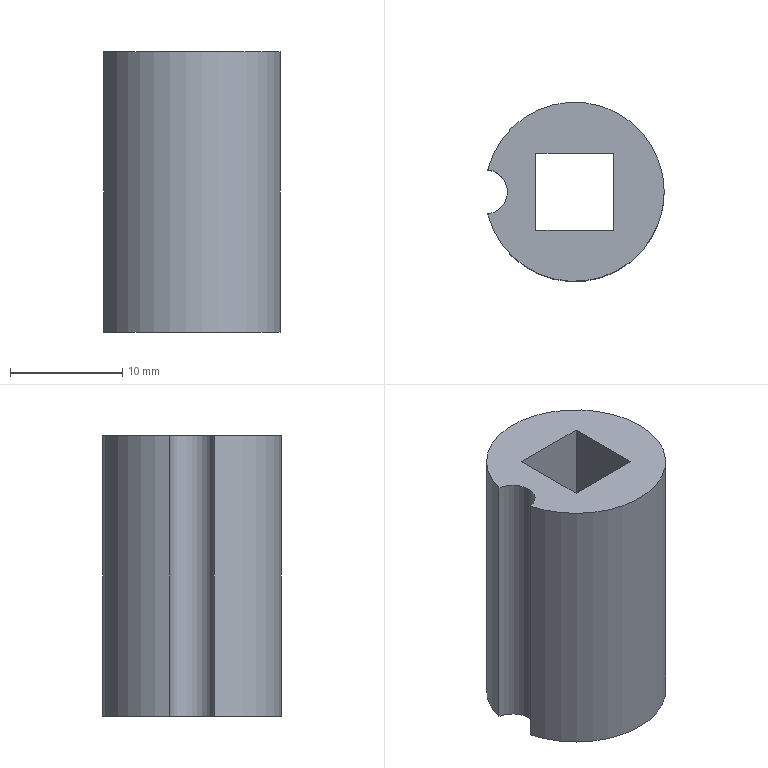Part | NX | features solid 2 | 1 solid | 10 faces | box 15.75 x 16 x 25 mm | volume 2997 mm3 | plane 7 | cylinder 3 | commonest cylinder face diameters 4 x1 10.6 x1 16 x1
STEP:
#1=CARTESIAN_POINT('',(705.26,-32.971,51.));
#2=VERTEX_POINT('',#1);
#3=CARTESIAN_POINT('',(705.26,-36.939,51.));
#4=VERTEX_POINT('',#3);
#5=CARTESIAN_POINT('',(705.01,-34.955,51.));
#6=DIRECTION('',(0.,0.,-1.));
#7=DIRECTION('',(1.,0.,0.));
#8=AXIS2_PLACEMENT_3D('',#5,#6,#7);
#9=CIRCLE('',#8,2.);
#10=EDGE_CURVE('',#2,#4,#9,.T.);
#11=ORIENTED_EDGE('',*,*,#10,.T.);
#12=CARTESIAN_POINT('',(713.01,-34.955,51.));
#13=DIRECTION('',(0.,0.,-1.));
#14=DIRECTION('',(1.,0.,0.));
#15=AXIS2_PLACEMENT_3D('',#12,#13,#14);
#16=CIRCLE('',#15,8.);
#17=EDGE_CURVE('',#2,#4,#16,.T.);
#18=ORIENTED_EDGE('',*,*,#17,.F.);
#19=EDGE_LOOP('',(#11,#18));
#20=FACE_BOUND('',#19,.T.);
#21=CARTESIAN_POINT('',(709.56,-31.505,51.));
#22=VERTEX_POINT('',#21);
#23=CARTESIAN_POINT('',(709.56,-38.405,51.));
#24=VERTEX_POINT('',#23);
#25=CARTESIAN_POINT('',(709.56,-34.955,51.));
#26=DIRECTION('',(0.,-1.,0.));
#27=VECTOR('',#26,1000.);
#28=LINE('',#25,#27);
#29=EDGE_CURVE('',#22,#24,#28,.T.);
#30=ORIENTED_EDGE('',*,*,#29,.F.);
#31=CARTESIAN_POINT('',(716.46,-31.505,51.));
#32=VERTEX_POINT('',#31);
#33=CARTESIAN_POINT('',(713.01,-31.505,51.));
#34=DIRECTION('',(1.,0.,0.));
#35=VECTOR('',#34,1000.);
#36=LINE('',#33,#35);
#37=EDGE_CURVE('',#22,#32,#36,.T.);
#38=ORIENTED_EDGE('',*,*,#37,.T.);
#39=CARTESIAN_POINT('',(716.46,-38.405,51.));
#40=VERTEX_POINT('',#39);
#41=CARTESIAN_POINT('',(716.46,-34.955,51.));
#42=DIRECTION('',(0.,-1.,0.));
#43=VECTOR('',#42,1000.);
#44=LINE('',#41,#43);
#45=EDGE_CURVE('',#32,#40,#44,.T.);
#46=ORIENTED_EDGE('',*,*,#45,.T.);
#47=CARTESIAN_POINT('',(713.01,-38.405,51.));
#48=DIRECTION('',(-1.,0.,0.));
#49=VECTOR('',#48,1000.);
#50=LINE('',#47,#49);
#51=EDGE_CURVE('',#40,#24,#50,.T.);
#52=ORIENTED_EDGE('',*,*,#51,.T.);
#53=EDGE_LOOP('',(#30,#38,#46,#52));
#54=FACE_BOUND('',#53,.T.);
#55=CARTESIAN_POINT('',(713.01,-34.955,51.));
#56=DIRECTION('',(0.,0.,1.));
#57=DIRECTION('',(-1.,0.,0.));
#58=AXIS2_PLACEMENT_3D('',#55,#56,#57);
#59=PLANE('',#58);
#60=ADVANCED_FACE('',(#20,#54),#59,.T.);
#61=CARTESIAN_POINT('',(705.26,-36.939,26.));
#62=VERTEX_POINT('',#61);
#63=CARTESIAN_POINT('',(705.26,-32.971,26.));
#64=VERTEX_POINT('',#63);
#65=CARTESIAN_POINT('',(705.01,-34.955,26.));
#66=DIRECTION('',(0.,0.,1.));
#67=DIRECTION('',(-1.,0.,0.));
#68=AXIS2_PLACEMENT_3D('',#65,#66,#67);
#69=CIRCLE('',#68,2.);
#70=EDGE_CURVE('',#62,#64,#69,.T.);
#71=ORIENTED_EDGE('',*,*,#70,.T.);
#72=CARTESIAN_POINT('',(713.01,-34.955,26.));
#73=DIRECTION('',(0.,0.,1.));
#74=DIRECTION('',(-1.,0.,0.));
#75=AXIS2_PLACEMENT_3D('',#72,#73,#74);
#76=CIRCLE('',#75,8.);
#77=EDGE_CURVE('',#62,#64,#76,.T.);
#78=ORIENTED_EDGE('',*,*,#77,.F.);
#79=EDGE_LOOP('',(#71,#78));
#80=FACE_BOUND('',#79,.T.);
#81=CARTESIAN_POINT('',(718.31,-34.955,26.));
#82=VERTEX_POINT('',#81);
#83=CARTESIAN_POINT('',(713.01,-34.955,26.));
#84=DIRECTION('',(0.,0.,-1.));
#85=DIRECTION('',(1.,0.,0.));
#86=AXIS2_PLACEMENT_3D('',#83,#84,#85);
#87=CIRCLE('',#86,5.3);
#88=EDGE_CURVE('',#82,#82,#87,.T.);
#89=ORIENTED_EDGE('',*,*,#88,.F.);
#90=EDGE_LOOP('',(#89));
#91=FACE_BOUND('',#90,.T.);
#92=CARTESIAN_POINT('',(713.01,-34.955,26.));
#93=DIRECTION('',(0.,0.,-1.));
#94=DIRECTION('',(1.,0.,0.));
#95=AXIS2_PLACEMENT_3D('',#92,#93,#94);
#96=PLANE('',#95);
#97=ADVANCED_FACE('',(#80,#91),#96,.T.);
#98=CARTESIAN_POINT('',(705.26,-32.971,38.5));
#99=DIRECTION('',(0.,0.,-1.));
#100=VECTOR('',#99,1000.);
#101=LINE('',#98,#100);
#102=EDGE_CURVE('',#2,#64,#101,.T.);
#103=ORIENTED_EDGE('',*,*,#102,.F.);
#104=ORIENTED_EDGE('',*,*,#17,.T.);
#105=CARTESIAN_POINT('',(705.26,-36.939,38.5));
#106=DIRECTION('',(0.,0.,-1.));
#107=VECTOR('',#106,1000.);
#108=LINE('',#105,#107);
#109=EDGE_CURVE('',#62,#4,#108,.F.);
#110=ORIENTED_EDGE('',*,*,#109,.F.);
#111=ORIENTED_EDGE('',*,*,#77,.T.);
#112=EDGE_LOOP('',(#103,#104,#110,#111));
#113=FACE_BOUND('',#112,.T.);
#114=CARTESIAN_POINT('',(713.01,-34.955,51.));
#115=DIRECTION('',(0.,0.,-1.));
#116=DIRECTION('',(1.,0.,0.));
#117=AXIS2_PLACEMENT_3D('',#114,#115,#116);
#118=CYLINDRICAL_SURFACE('',#117,8.);
#119=ADVANCED_FACE('',(#113),#118,.T.);
#120=CARTESIAN_POINT('',(716.46,-31.505,43.));
#121=VERTEX_POINT('',#120);
#122=CARTESIAN_POINT('',(709.56,-31.505,43.));
#123=VERTEX_POINT('',#122);
#124=CARTESIAN_POINT('',(716.46,-31.505,43.));
#125=DIRECTION('',(-1.,0.,0.));
#126=VECTOR('',#125,1000.);
#127=LINE('',#124,#126);
#128=EDGE_CURVE('',#121,#123,#127,.T.);
#129=ORIENTED_EDGE('',*,*,#128,.F.);
#130=CARTESIAN_POINT('',(716.46,-31.505,56.));
#131=DIRECTION('',(0.,0.,-1.));
#132=VECTOR('',#131,1000.);
#133=LINE('',#130,#132);
#134=EDGE_CURVE('',#32,#121,#133,.T.);
#135=ORIENTED_EDGE('',*,*,#134,.F.);
#136=ORIENTED_EDGE('',*,*,#37,.F.);
#137=CARTESIAN_POINT('',(709.56,-31.505,56.));
#138=DIRECTION('',(0.,0.,-1.));
#139=VECTOR('',#138,1000.);
#140=LINE('',#137,#139);
#141=EDGE_CURVE('',#22,#123,#140,.T.);
#142=ORIENTED_EDGE('',*,*,#141,.T.);
#143=EDGE_LOOP('',(#129,#135,#136,#142));
#144=FACE_BOUND('',#143,.T.);
#145=CARTESIAN_POINT('',(716.46,-31.505,56.));
#146=DIRECTION('',(0.,-1.,0.));
#147=DIRECTION('',(0.,0.,1.));
#148=AXIS2_PLACEMENT_3D('',#145,#146,#147);
#149=PLANE('',#148);
#150=ADVANCED_FACE('',(#144),#149,.T.);
#151=CARTESIAN_POINT('',(709.56,-38.405,43.));
#152=VERTEX_POINT('',#151);
#153=CARTESIAN_POINT('',(709.56,-38.405,56.));
#154=DIRECTION('',(0.,0.,-1.));
#155=VECTOR('',#154,1000.);
#156=LINE('',#153,#155);
#157=EDGE_CURVE('',#24,#152,#156,.T.);
#158=ORIENTED_EDGE('',*,*,#157,.T.);
#159=CARTESIAN_POINT('',(709.56,-38.405,43.));
#160=DIRECTION('',(0.,1.,0.));
#161=VECTOR('',#160,1000.);
#162=LINE('',#159,#161);
#163=EDGE_CURVE('',#152,#123,#162,.T.);
#164=ORIENTED_EDGE('',*,*,#163,.T.);
#165=ORIENTED_EDGE('',*,*,#141,.F.);
#166=ORIENTED_EDGE('',*,*,#29,.T.);
#167=EDGE_LOOP('',(#158,#164,#165,#166));
#168=FACE_BOUND('',#167,.T.);
#169=CARTESIAN_POINT('',(709.56,-38.405,56.));
#170=DIRECTION('',(-1.,0.,0.));
#171=DIRECTION('',(0.,0.,-1.));
#172=AXIS2_PLACEMENT_3D('',#169,#170,#171);
#173=PLANE('',#172);
#174=ADVANCED_FACE('',(#168),#173,.F.);
#175=CARTESIAN_POINT('',(716.46,-38.405,43.));
#176=VERTEX_POINT('',#175);
#177=CARTESIAN_POINT('',(709.56,-38.405,43.));
#178=DIRECTION('',(1.,0.,0.));
#179=VECTOR('',#178,1000.);
#180=LINE('',#177,#179);
#181=EDGE_CURVE('',#152,#176,#180,.T.);
#182=ORIENTED_EDGE('',*,*,#181,.F.);
#183=ORIENTED_EDGE('',*,*,#157,.F.);
#184=ORIENTED_EDGE('',*,*,#51,.F.);
#185=CARTESIAN_POINT('',(716.46,-38.405,56.));
#186=DIRECTION('',(0.,0.,-1.));
#187=VECTOR('',#186,1000.);
#188=LINE('',#185,#187);
#189=EDGE_CURVE('',#40,#176,#188,.T.);
#190=ORIENTED_EDGE('',*,*,#189,.T.);
#191=EDGE_LOOP('',(#182,#183,#184,#190));
#192=FACE_BOUND('',#191,.T.);
#193=CARTESIAN_POINT('',(709.56,-38.405,56.));
#194=DIRECTION('',(0.,1.,0.));
#195=DIRECTION('',(0.,0.,-1.));
#196=AXIS2_PLACEMENT_3D('',#193,#194,#195);
#197=PLANE('',#196);
#198=ADVANCED_FACE('',(#192),#197,.T.);
#199=CARTESIAN_POINT('',(716.46,-38.405,43.));
#200=DIRECTION('',(0.,1.,0.));
#201=VECTOR('',#200,1000.);
#202=LINE('',#199,#201);
#203=EDGE_CURVE('',#176,#121,#202,.T.);
#204=ORIENTED_EDGE('',*,*,#203,.F.);
#205=ORIENTED_EDGE('',*,*,#189,.F.);
#206=ORIENTED_EDGE('',*,*,#45,.F.);
#207=ORIENTED_EDGE('',*,*,#134,.T.);
#208=EDGE_LOOP('',(#204,#205,#206,#207));
#209=FACE_BOUND('',#208,.T.);
#210=CARTESIAN_POINT('',(716.46,-38.405,56.));
#211=DIRECTION('',(-1.,0.,0.));
#212=DIRECTION('',(0.,0.,-1.));
#213=AXIS2_PLACEMENT_3D('',#210,#211,#212);
#214=PLANE('',#213);
#215=ADVANCED_FACE('',(#209),#214,.T.);
#216=ORIENTED_EDGE('',*,*,#128,.T.);
#217=ORIENTED_EDGE('',*,*,#163,.F.);
#218=ORIENTED_EDGE('',*,*,#181,.T.);
#219=ORIENTED_EDGE('',*,*,#203,.T.);
#220=EDGE_LOOP('',(#216,#217,#218,#219));
#221=FACE_BOUND('',#220,.T.);
#222=CARTESIAN_POINT('',(718.31,-34.955,43.));
#223=VERTEX_POINT('',#222);
#224=CARTESIAN_POINT('',(713.01,-34.955,43.));
#225=DIRECTION('',(0.,0.,-1.));
#226=DIRECTION('',(1.,0.,0.));
#227=AXIS2_PLACEMENT_3D('',#224,#225,#226);
#228=CIRCLE('',#227,5.3);
#229=EDGE_CURVE('',#223,#223,#228,.T.);
#230=ORIENTED_EDGE('',*,*,#229,.T.);
#231=EDGE_LOOP('',(#230));
#232=FACE_BOUND('',#231,.T.);
#233=CARTESIAN_POINT('',(713.01,-34.955,43.));
#234=DIRECTION('',(0.,0.,1.));
#235=DIRECTION('',(-1.,0.,0.));
#236=AXIS2_PLACEMENT_3D('',#233,#234,#235);
#237=PLANE('',#236);
#238=ADVANCED_FACE('',(#221,#232),#237,.F.);
#239=ORIENTED_EDGE('',*,*,#88,.T.);
#240=EDGE_LOOP('',(#239));
#241=FACE_BOUND('',#240,.T.);
#242=ORIENTED_EDGE('',*,*,#229,.F.);
#243=EDGE_LOOP('',(#242));
#244=FACE_BOUND('',#243,.T.);
#245=CARTESIAN_POINT('',(713.01,-34.955,43.));
#246=DIRECTION('',(0.,0.,-1.));
#247=DIRECTION('',(1.,0.,0.));
#248=AXIS2_PLACEMENT_3D('',#245,#246,#247);
#249=CYLINDRICAL_SURFACE('',#248,5.3);
#250=ADVANCED_FACE('',(#241,#244),#249,.F.);
#251=ORIENTED_EDGE('',*,*,#102,.T.);
#252=ORIENTED_EDGE('',*,*,#70,.F.);
#253=ORIENTED_EDGE('',*,*,#109,.T.);
#254=ORIENTED_EDGE('',*,*,#10,.F.);
#255=EDGE_LOOP('',(#251,#252,#253,#254));
#256=FACE_BOUND('',#255,.T.);
#257=CARTESIAN_POINT('',(705.01,-34.955,51.));
#258=DIRECTION('',(0.,0.,-1.));
#259=DIRECTION('',(1.,0.,0.));
#260=AXIS2_PLACEMENT_3D('',#257,#258,#259);
#261=CYLINDRICAL_SURFACE('',#260,2.);
#262=ADVANCED_FACE('',(#256),#261,.F.);
#263=CLOSED_SHELL('',(#60,#97,#119,#150,#174,#198,#215,#238,#250,#262));
#264=MANIFOLD_SOLID_BREP('',#263);
#265=(LENGTH_UNIT()NAMED_UNIT(*)SI_UNIT(.MILLI.,.METRE.));
#266=UNCERTAINTY_MEASURE_WITH_UNIT(LENGTH_MEASURE(0.00001),#265,'','');
#267=(NAMED_UNIT(*)PLANE_ANGLE_UNIT()SI_UNIT($,.RADIAN.));
#268=(NAMED_UNIT(*)SI_UNIT($,.STERADIAN.)SOLID_ANGLE_UNIT());
#269=(GEOMETRIC_REPRESENTATION_CONTEXT(3)GLOBAL_UNCERTAINTY_ASSIGNED_CONTEXT((#266))GLOBAL_UNIT_ASSIGNED_CONTEXT((#265,#267,#268))REPRESENTATION_CONTEXT('',''));
#270=ADVANCED_BREP_SHAPE_REPRESENTATION('',(#264),#269);